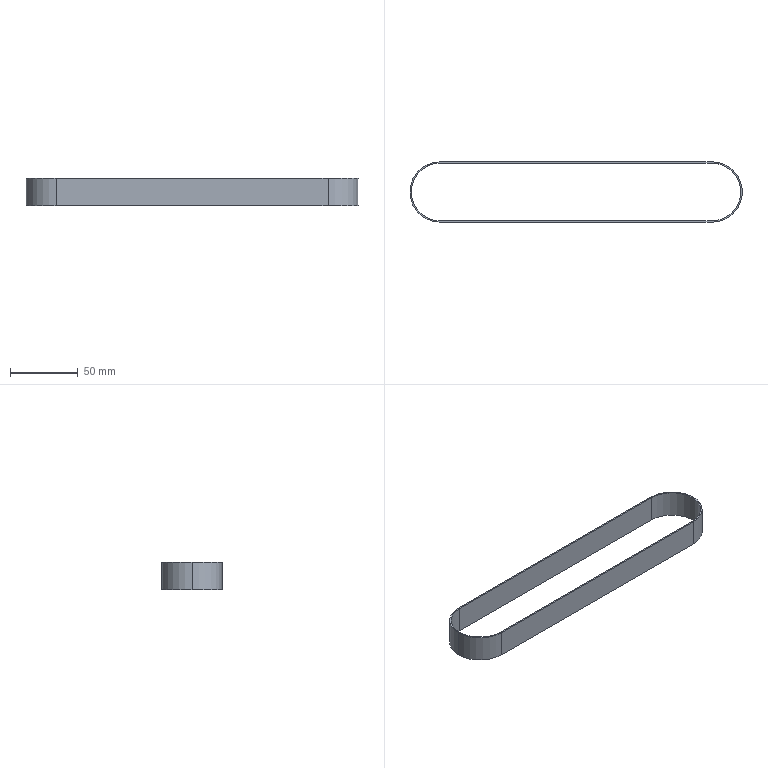Part | STEP file | PN_0049 (timing belt 210L, W20, Z=56) | 1 solid | 12 faces | box 244.45 x 44.45 x 20 mm | volume 10730 mm3 | cylinder 6 | plane 6 | commonest cylinder face diameters 42.45 x3 44.45 x3
STEP:
#1=CARTESIAN_POINT('',(0.,0.,0.));
#2=DIRECTION('',(0.,0.,1.));
#3=DIRECTION('',(1.,0.,0.));
#4=AXIS2_PLACEMENT_3D('',#1,#2,#3);
#5=CARTESIAN_POINT('',(-100.,21.225,10.));
#6=VERTEX_POINT('',#5);
#7=CARTESIAN_POINT('',(-100.,21.225,-10.));
#8=VERTEX_POINT('',#7);
#9=CARTESIAN_POINT('',(-100.,21.225,10.));
#10=DIRECTION('',(0.,0.,-1.));
#11=VECTOR('',#10,1.);
#12=LINE('',#9,#11);
#13=CARTESIAN_POINT('',(-100.,0.,10.));
#14=DIRECTION('',(0.,0.,-1.));
#15=DIRECTION('',(-1.,0.,0.));
#16=AXIS2_PLACEMENT_3D('',#13,#14,#15);
#17=CYLINDRICAL_SURFACE('',#16,21.225);
#18=CARTESIAN_POINT('',(1.571,0.));
#19=DIRECTION('',(0.,1.));
#20=VECTOR('',#19,1.);
#21=LINE('',#18,#20);
#22=(GEOMETRIC_REPRESENTATION_CONTEXT(2)PARAMETRIC_REPRESENTATION_CONTEXT()REPRESENTATION_CONTEXT('',''));
#23=DEFINITIONAL_REPRESENTATION('',(#21),#22);
#24=PCURVE('',#17,#23);
#25=CARTESIAN_POINT('',(-100.,21.225,10.));
#26=DIRECTION('',(0.,-1.,0.));
#27=DIRECTION('',(0.,0.,-1.));
#28=AXIS2_PLACEMENT_3D('',#25,#26,#27);
#29=PLANE('',#28);
#30=CARTESIAN_POINT('',(0.,0.));
#31=DIRECTION('',(1.,0.));
#32=VECTOR('',#31,1.);
#33=LINE('',#30,#32);
#34=(GEOMETRIC_REPRESENTATION_CONTEXT(2)PARAMETRIC_REPRESENTATION_CONTEXT()REPRESENTATION_CONTEXT('',''));
#35=DEFINITIONAL_REPRESENTATION('',(#33),#34);
#36=PCURVE('',#29,#35);
#37=SURFACE_CURVE('',#12,(#24,#36),.PCURVE_S1.);
#38=EDGE_CURVE('',#6,#8,#37,.T.);
#39=ORIENTED_EDGE('',*,*,#38,.T.);
#40=CARTESIAN_POINT('',(-121.225,0.,-10.));
#41=VERTEX_POINT('',#40);
#42=CARTESIAN_POINT('',(-100.,0.,-10.));
#43=DIRECTION('',(0.,0.,1.));
#44=DIRECTION('',(1.,0.,0.));
#45=AXIS2_PLACEMENT_3D('',#42,#43,#44);
#46=CIRCLE('',#45,21.225);
#47=CARTESIAN_POINT('',(3.142,20.));
#48=DIRECTION('',(-1.,0.));
#49=VECTOR('',#48,1.);
#50=LINE('',#47,#49);
#51=(GEOMETRIC_REPRESENTATION_CONTEXT(2)PARAMETRIC_REPRESENTATION_CONTEXT()REPRESENTATION_CONTEXT('',''));
#52=DEFINITIONAL_REPRESENTATION('',(#50),#51);
#53=PCURVE('',#17,#52);
#54=CARTESIAN_POINT('',(-100.,0.,-10.));
#55=DIRECTION('',(0.,0.,1.));
#56=DIRECTION('',(1.,0.,0.));
#57=AXIS2_PLACEMENT_3D('',#54,#55,#56);
#58=PLANE('',#57);
#59=CARTESIAN_POINT('',(0.,0.));
#60=DIRECTION('',(1.,0.));
#61=AXIS2_PLACEMENT_2D('',#59,#60);
#62=CIRCLE('',#61,21.225);
#63=(GEOMETRIC_REPRESENTATION_CONTEXT(2)PARAMETRIC_REPRESENTATION_CONTEXT()REPRESENTATION_CONTEXT('',''));
#64=DEFINITIONAL_REPRESENTATION('',(#62),#63);
#65=PCURVE('',#58,#64);
#66=SURFACE_CURVE('',#46,(#53,#65),.PCURVE_S1.);
#67=EDGE_CURVE('',#8,#41,#66,.T.);
#68=ORIENTED_EDGE('',*,*,#67,.T.);
#69=CARTESIAN_POINT('',(-121.225,0.,10.));
#70=VERTEX_POINT('',#69);
#71=CARTESIAN_POINT('',(-121.225,0.,10.));
#72=DIRECTION('',(0.,0.,-1.));
#73=VECTOR('',#72,1.);
#74=LINE('',#71,#73);
#75=CARTESIAN_POINT('',(0.,0.));
#76=DIRECTION('',(0.,1.));
#77=VECTOR('',#76,1.);
#78=LINE('',#75,#77);
#79=(GEOMETRIC_REPRESENTATION_CONTEXT(2)PARAMETRIC_REPRESENTATION_CONTEXT()REPRESENTATION_CONTEXT('',''));
#80=DEFINITIONAL_REPRESENTATION('',(#78),#79);
#81=PCURVE('',#17,#80);
#82=CARTESIAN_POINT('',(-100.,0.,10.));
#83=DIRECTION('',(0.,0.,-1.));
#84=DIRECTION('',(-1.,0.,0.));
#85=AXIS2_PLACEMENT_3D('',#82,#83,#84);
#86=CYLINDRICAL_SURFACE('',#85,21.225);
#87=CARTESIAN_POINT('',(6.283,0.));
#88=DIRECTION('',(0.,1.));
#89=VECTOR('',#88,1.);
#90=LINE('',#87,#89);
#91=(GEOMETRIC_REPRESENTATION_CONTEXT(2)PARAMETRIC_REPRESENTATION_CONTEXT()REPRESENTATION_CONTEXT('',''));
#92=DEFINITIONAL_REPRESENTATION('',(#90),#91);
#93=PCURVE('',#86,#92);
#94=SURFACE_CURVE('',#74,(#81,#93),.PCURVE_S1.);
#95=EDGE_CURVE('',#70,#41,#94,.T.);
#96=ORIENTED_EDGE('',*,*,#95,.F.);
#97=CARTESIAN_POINT('',(-100.,0.,10.));
#98=DIRECTION('',(0.,0.,1.));
#99=DIRECTION('',(1.,0.,0.));
#100=AXIS2_PLACEMENT_3D('',#97,#98,#99);
#101=CIRCLE('',#100,21.225);
#102=CARTESIAN_POINT('',(3.142,0.));
#103=DIRECTION('',(-1.,0.));
#104=VECTOR('',#103,1.);
#105=LINE('',#102,#104);
#106=(GEOMETRIC_REPRESENTATION_CONTEXT(2)PARAMETRIC_REPRESENTATION_CONTEXT()REPRESENTATION_CONTEXT('',''));
#107=DEFINITIONAL_REPRESENTATION('',(#105),#106);
#108=PCURVE('',#17,#107);
#109=CARTESIAN_POINT('',(-100.,0.,10.));
#110=DIRECTION('',(0.,0.,1.));
#111=DIRECTION('',(1.,0.,0.));
#112=AXIS2_PLACEMENT_3D('',#109,#110,#111);
#113=PLANE('',#112);
#114=CARTESIAN_POINT('',(0.,0.));
#115=DIRECTION('',(1.,0.));
#116=AXIS2_PLACEMENT_2D('',#114,#115);
#117=CIRCLE('',#116,21.225);
#118=(GEOMETRIC_REPRESENTATION_CONTEXT(2)PARAMETRIC_REPRESENTATION_CONTEXT()REPRESENTATION_CONTEXT('',''));
#119=DEFINITIONAL_REPRESENTATION('',(#117),#118);
#120=PCURVE('',#113,#119);
#121=SURFACE_CURVE('',#101,(#108,#120),.PCURVE_S1.);
#122=EDGE_CURVE('',#6,#70,#121,.T.);
#123=ORIENTED_EDGE('',*,*,#122,.F.);
#124=EDGE_LOOP('',(#39,#68,#96,#123));
#125=FACE_BOUND('',#124,.F.);
#126=ADVANCED_FACE('',(#125),#17,.F.);
#127=CARTESIAN_POINT('',(-122.225,0.,10.));
#128=VERTEX_POINT('',#127);
#129=CARTESIAN_POINT('',(-100.,-22.225,10.));
#130=VERTEX_POINT('',#129);
#131=CARTESIAN_POINT('',(-100.,0.,10.));
#132=DIRECTION('',(0.,0.,1.));
#133=DIRECTION('',(1.,0.,0.));
#134=AXIS2_PLACEMENT_3D('',#131,#132,#133);
#135=CIRCLE('',#134,22.225);
#136=CARTESIAN_POINT('',(-100.,0.,10.));
#137=DIRECTION('',(0.,0.,-1.));
#138=DIRECTION('',(-1.,0.,0.));
#139=AXIS2_PLACEMENT_3D('',#136,#137,#138);
#140=CYLINDRICAL_SURFACE('',#139,22.225);
#141=CARTESIAN_POINT('',(9.425,0.));
#142=DIRECTION('',(-1.,0.));
#143=VECTOR('',#142,1.);
#144=LINE('',#141,#143);
#145=(GEOMETRIC_REPRESENTATION_CONTEXT(2)PARAMETRIC_REPRESENTATION_CONTEXT()REPRESENTATION_CONTEXT('',''));
#146=DEFINITIONAL_REPRESENTATION('',(#144),#145);
#147=PCURVE('',#140,#146);
#148=CARTESIAN_POINT('',(0.,0.));
#149=DIRECTION('',(1.,0.));
#150=AXIS2_PLACEMENT_2D('',#148,#149);
#151=CIRCLE('',#150,22.225);
#152=(GEOMETRIC_REPRESENTATION_CONTEXT(2)PARAMETRIC_REPRESENTATION_CONTEXT()REPRESENTATION_CONTEXT('',''));
#153=DEFINITIONAL_REPRESENTATION('',(#151),#152);
#154=PCURVE('',#113,#153);
#155=SURFACE_CURVE('',#135,(#147,#154),.PCURVE_S1.);
#156=EDGE_CURVE('',#128,#130,#155,.T.);
#157=ORIENTED_EDGE('',*,*,#156,.F.);
#158=CARTESIAN_POINT('',(-122.225,0.,-10.));
#159=VERTEX_POINT('',#158);
#160=CARTESIAN_POINT('',(-122.225,0.,10.));
#161=DIRECTION('',(0.,0.,-1.));
#162=VECTOR('',#161,1.);
#163=LINE('',#160,#162);
#164=CARTESIAN_POINT('',(6.283,0.));
#165=DIRECTION('',(0.,1.));
#166=VECTOR('',#165,1.);
#167=LINE('',#164,#166);
#168=(GEOMETRIC_REPRESENTATION_CONTEXT(2)PARAMETRIC_REPRESENTATION_CONTEXT()REPRESENTATION_CONTEXT('',''));
#169=DEFINITIONAL_REPRESENTATION('',(#167),#168);
#170=PCURVE('',#140,#169);
#171=CARTESIAN_POINT('',(-100.,0.,10.));
#172=DIRECTION('',(0.,0.,-1.));
#173=DIRECTION('',(-1.,0.,0.));
#174=AXIS2_PLACEMENT_3D('',#171,#172,#173);
#175=CYLINDRICAL_SURFACE('',#174,22.225);
#176=CARTESIAN_POINT('',(0.,0.));
#177=DIRECTION('',(0.,1.));
#178=VECTOR('',#177,1.);
#179=LINE('',#176,#178);
#180=(GEOMETRIC_REPRESENTATION_CONTEXT(2)PARAMETRIC_REPRESENTATION_CONTEXT()REPRESENTATION_CONTEXT('',''));
#181=DEFINITIONAL_REPRESENTATION('',(#179),#180);
#182=PCURVE('',#175,#181);
#183=SURFACE_CURVE('',#163,(#170,#182),.PCURVE_S1.);
#184=EDGE_CURVE('',#128,#159,#183,.T.);
#185=ORIENTED_EDGE('',*,*,#184,.T.);
#186=CARTESIAN_POINT('',(-100.,-22.225,-10.));
#187=VERTEX_POINT('',#186);
#188=CARTESIAN_POINT('',(-100.,0.,-10.));
#189=DIRECTION('',(0.,0.,1.));
#190=DIRECTION('',(1.,0.,0.));
#191=AXIS2_PLACEMENT_3D('',#188,#189,#190);
#192=CIRCLE('',#191,22.225);
#193=CARTESIAN_POINT('',(9.425,20.));
#194=DIRECTION('',(-1.,0.));
#195=VECTOR('',#194,1.);
#196=LINE('',#193,#195);
#197=(GEOMETRIC_REPRESENTATION_CONTEXT(2)PARAMETRIC_REPRESENTATION_CONTEXT()REPRESENTATION_CONTEXT('',''));
#198=DEFINITIONAL_REPRESENTATION('',(#196),#197);
#199=PCURVE('',#140,#198);
#200=CARTESIAN_POINT('',(0.,0.));
#201=DIRECTION('',(1.,0.));
#202=AXIS2_PLACEMENT_2D('',#200,#201);
#203=CIRCLE('',#202,22.225);
#204=(GEOMETRIC_REPRESENTATION_CONTEXT(2)PARAMETRIC_REPRESENTATION_CONTEXT()REPRESENTATION_CONTEXT('',''));
#205=DEFINITIONAL_REPRESENTATION('',(#203),#204);
#206=PCURVE('',#58,#205);
#207=SURFACE_CURVE('',#192,(#199,#206),.PCURVE_S1.);
#208=EDGE_CURVE('',#159,#187,#207,.T.);
#209=ORIENTED_EDGE('',*,*,#208,.T.);
#210=CARTESIAN_POINT('',(-100.,-22.225,10.));
#211=DIRECTION('',(0.,0.,-1.));
#212=VECTOR('',#211,1.);
#213=LINE('',#210,#212);
#214=CARTESIAN_POINT('',(4.712,0.));
#215=DIRECTION('',(0.,1.));
#216=VECTOR('',#215,1.);
#217=LINE('',#214,#216);
#218=(GEOMETRIC_REPRESENTATION_CONTEXT(2)PARAMETRIC_REPRESENTATION_CONTEXT()REPRESENTATION_CONTEXT('',''));
#219=DEFINITIONAL_REPRESENTATION('',(#217),#218);
#220=PCURVE('',#140,#219);
#221=CARTESIAN_POINT('',(-100.,-22.225,10.));
#222=DIRECTION('',(0.,1.,0.));
#223=DIRECTION('',(0.,0.,1.));
#224=AXIS2_PLACEMENT_3D('',#221,#222,#223);
#225=PLANE('',#224);
#226=CARTESIAN_POINT('',(0.,0.));
#227=DIRECTION('',(-1.,0.));
#228=VECTOR('',#227,1.);
#229=LINE('',#226,#228);
#230=(GEOMETRIC_REPRESENTATION_CONTEXT(2)PARAMETRIC_REPRESENTATION_CONTEXT()REPRESENTATION_CONTEXT('',''));
#231=DEFINITIONAL_REPRESENTATION('',(#229),#230);
#232=PCURVE('',#225,#231);
#233=SURFACE_CURVE('',#213,(#220,#232),.PCURVE_S1.);
#234=EDGE_CURVE('',#130,#187,#233,.T.);
#235=ORIENTED_EDGE('',*,*,#234,.F.);
#236=EDGE_LOOP('',(#157,#185,#209,#235));
#237=FACE_BOUND('',#236,.T.);
#238=ADVANCED_FACE('',(#237),#140,.T.);
#239=CARTESIAN_POINT('',(-100.,22.225,10.));
#240=VERTEX_POINT('',#239);
#241=CARTESIAN_POINT('',(-100.,0.,10.));
#242=DIRECTION('',(0.,0.,1.));
#243=DIRECTION('',(1.,0.,0.));
#244=AXIS2_PLACEMENT_3D('',#241,#242,#243);
#245=CIRCLE('',#244,22.225);
#246=CARTESIAN_POINT('',(0.,0.));
#247=DIRECTION('',(1.,0.));
#248=AXIS2_PLACEMENT_2D('',#246,#247);
#249=CIRCLE('',#248,22.225);
#250=(GEOMETRIC_REPRESENTATION_CONTEXT(2)PARAMETRIC_REPRESENTATION_CONTEXT()REPRESENTATION_CONTEXT('',''));
#251=DEFINITIONAL_REPRESENTATION('',(#249),#250);
#252=PCURVE('',#113,#251);
#253=CARTESIAN_POINT('',(3.142,0.));
#254=DIRECTION('',(-1.,0.));
#255=VECTOR('',#254,1.);
#256=LINE('',#253,#255);
#257=(GEOMETRIC_REPRESENTATION_CONTEXT(2)PARAMETRIC_REPRESENTATION_CONTEXT()REPRESENTATION_CONTEXT('',''));
#258=DEFINITIONAL_REPRESENTATION('',(#256),#257);
#259=PCURVE('',#175,#258);
#260=SURFACE_CURVE('',#245,(#252,#259),.PCURVE_S1.);
#261=EDGE_CURVE('',#240,#128,#260,.T.);
#262=ORIENTED_EDGE('',*,*,#261,.T.);
#263=ORIENTED_EDGE('',*,*,#156,.T.);
#264=CARTESIAN_POINT('',(100.,-22.225,10.));
#265=VERTEX_POINT('',#264);
#266=CARTESIAN_POINT('',(-100.,-22.225,10.));
#267=DIRECTION('',(1.,0.,0.));
#268=VECTOR('',#267,1.);
#269=LINE('',#266,#268);
#270=CARTESIAN_POINT('',(0.,-22.225));
#271=DIRECTION('',(1.,0.));
#272=VECTOR('',#271,1.);
#273=LINE('',#270,#272);
#274=(GEOMETRIC_REPRESENTATION_CONTEXT(2)PARAMETRIC_REPRESENTATION_CONTEXT()REPRESENTATION_CONTEXT('',''));
#275=DEFINITIONAL_REPRESENTATION('',(#273),#274);
#276=PCURVE('',#113,#275);
#277=CARTESIAN_POINT('',(0.,0.));
#278=DIRECTION('',(0.,1.));
#279=VECTOR('',#278,1.);
#280=LINE('',#277,#279);
#281=(GEOMETRIC_REPRESENTATION_CONTEXT(2)PARAMETRIC_REPRESENTATION_CONTEXT()REPRESENTATION_CONTEXT('',''));
#282=DEFINITIONAL_REPRESENTATION('',(#280),#281);
#283=PCURVE('',#225,#282);
#284=SURFACE_CURVE('',#269,(#276,#283),.PCURVE_S1.);
#285=EDGE_CURVE('',#130,#265,#284,.T.);
#286=ORIENTED_EDGE('',*,*,#285,.T.);
#287=CARTESIAN_POINT('',(100.,22.225,10.));
#288=VERTEX_POINT('',#287);
#289=CARTESIAN_POINT('',(100.,0.,10.));
#290=DIRECTION('',(0.,0.,1.));
#291=DIRECTION('',(1.,0.,0.));
#292=AXIS2_PLACEMENT_3D('',#289,#290,#291);
#293=CIRCLE('',#292,22.225);
#294=CARTESIAN_POINT('',(200.,0.));
#295=DIRECTION('',(1.,0.));
#296=AXIS2_PLACEMENT_2D('',#294,#295);
#297=CIRCLE('',#296,22.225);
#298=(GEOMETRIC_REPRESENTATION_CONTEXT(2)PARAMETRIC_REPRESENTATION_CONTEXT()REPRESENTATION_CONTEXT('',''));
#299=DEFINITIONAL_REPRESENTATION('',(#297),#298);
#300=PCURVE('',#113,#299);
#301=CARTESIAN_POINT('',(100.,0.,10.));
#302=DIRECTION('',(0.,0.,-1.));
#303=DIRECTION('',(-1.,0.,0.));
#304=AXIS2_PLACEMENT_3D('',#301,#302,#303);
#305=CYLINDRICAL_SURFACE('',#304,22.225);
#306=CARTESIAN_POINT('',(9.425,0.));
#307=DIRECTION('',(-1.,0.));
#308=VECTOR('',#307,1.);
#309=LINE('',#306,#308);
#310=(GEOMETRIC_REPRESENTATION_CONTEXT(2)PARAMETRIC_REPRESENTATION_CONTEXT()REPRESENTATION_CONTEXT('',''));
#311=DEFINITIONAL_REPRESENTATION('',(#309),#310);
#312=PCURVE('',#305,#311);
#313=SURFACE_CURVE('',#293,(#300,#312),.PCURVE_S1.);
#314=EDGE_CURVE('',#265,#288,#313,.T.);
#315=ORIENTED_EDGE('',*,*,#314,.T.);
#316=CARTESIAN_POINT('',(-100.,22.225,10.));
#317=DIRECTION('',(-1.,0.,0.));
#318=VECTOR('',#317,1.);
#319=LINE('',#316,#318);
#320=CARTESIAN_POINT('',(0.,22.225));
#321=DIRECTION('',(-1.,0.));
#322=VECTOR('',#321,1.);
#323=LINE('',#320,#322);
#324=(GEOMETRIC_REPRESENTATION_CONTEXT(2)PARAMETRIC_REPRESENTATION_CONTEXT()REPRESENTATION_CONTEXT('',''));
#325=DEFINITIONAL_REPRESENTATION('',(#323),#324);
#326=PCURVE('',#113,#325);
#327=CARTESIAN_POINT('',(-100.,22.225,10.));
#328=DIRECTION('',(0.,-1.,0.));
#329=DIRECTION('',(0.,0.,-1.));
#330=AXIS2_PLACEMENT_3D('',#327,#328,#329);
#331=PLANE('',#330);
#332=CARTESIAN_POINT('',(0.,0.));
#333=DIRECTION('',(0.,-1.));
#334=VECTOR('',#333,1.);
#335=LINE('',#332,#334);
#336=(GEOMETRIC_REPRESENTATION_CONTEXT(2)PARAMETRIC_REPRESENTATION_CONTEXT()REPRESENTATION_CONTEXT('',''));
#337=DEFINITIONAL_REPRESENTATION('',(#335),#336);
#338=PCURVE('',#331,#337);
#339=SURFACE_CURVE('',#319,(#326,#338),.PCURVE_S1.);
#340=EDGE_CURVE('',#288,#240,#339,.T.);
#341=ORIENTED_EDGE('',*,*,#340,.T.);
#342=EDGE_LOOP('',(#262,#263,#286,#315,#341));
#343=FACE_BOUND('',#342,.T.);
#344=CARTESIAN_POINT('',(-100.,-21.225,10.));
#345=VERTEX_POINT('',#344);
#346=CARTESIAN_POINT('',(100.,-21.225,10.));
#347=VERTEX_POINT('',#346);
#348=CARTESIAN_POINT('',(-100.,-21.225,10.));
#349=DIRECTION('',(1.,0.,0.));
#350=VECTOR('',#349,1.);
#351=LINE('',#348,#350);
#352=CARTESIAN_POINT('',(0.,-21.225));
#353=DIRECTION('',(1.,0.));
#354=VECTOR('',#353,1.);
#355=LINE('',#352,#354);
#356=(GEOMETRIC_REPRESENTATION_CONTEXT(2)PARAMETRIC_REPRESENTATION_CONTEXT()REPRESENTATION_CONTEXT('',''));
#357=DEFINITIONAL_REPRESENTATION('',(#355),#356);
#358=PCURVE('',#113,#357);
#359=CARTESIAN_POINT('',(-100.,-21.225,10.));
#360=DIRECTION('',(0.,1.,0.));
#361=DIRECTION('',(0.,0.,1.));
#362=AXIS2_PLACEMENT_3D('',#359,#360,#361);
#363=PLANE('',#362);
#364=CARTESIAN_POINT('',(0.,0.));
#365=DIRECTION('',(0.,1.));
#366=VECTOR('',#365,1.);
#367=LINE('',#364,#366);
#368=(GEOMETRIC_REPRESENTATION_CONTEXT(2)PARAMETRIC_REPRESENTATION_CONTEXT()REPRESENTATION_CONTEXT('',''));
#369=DEFINITIONAL_REPRESENTATION('',(#367),#368);
#370=PCURVE('',#363,#369);
#371=SURFACE_CURVE('',#351,(#358,#370),.PCURVE_S1.);
#372=EDGE_CURVE('',#345,#347,#371,.T.);
#373=ORIENTED_EDGE('',*,*,#372,.F.);
#374=CARTESIAN_POINT('',(-100.,0.,10.));
#375=DIRECTION('',(0.,0.,1.));
#376=DIRECTION('',(1.,0.,0.));
#377=AXIS2_PLACEMENT_3D('',#374,#375,#376);
#378=CIRCLE('',#377,21.225);
#379=CARTESIAN_POINT('',(0.,0.));
#380=DIRECTION('',(1.,0.));
#381=AXIS2_PLACEMENT_2D('',#379,#380);
#382=CIRCLE('',#381,21.225);
#383=(GEOMETRIC_REPRESENTATION_CONTEXT(2)PARAMETRIC_REPRESENTATION_CONTEXT()REPRESENTATION_CONTEXT('',''));
#384=DEFINITIONAL_REPRESENTATION('',(#382),#383);
#385=PCURVE('',#113,#384);
#386=CARTESIAN_POINT('',(9.425,0.));
#387=DIRECTION('',(-1.,0.));
#388=VECTOR('',#387,1.);
#389=LINE('',#386,#388);
#390=(GEOMETRIC_REPRESENTATION_CONTEXT(2)PARAMETRIC_REPRESENTATION_CONTEXT()REPRESENTATION_CONTEXT('',''));
#391=DEFINITIONAL_REPRESENTATION('',(#389),#390);
#392=PCURVE('',#86,#391);
#393=SURFACE_CURVE('',#378,(#385,#392),.PCURVE_S1.);
#394=EDGE_CURVE('',#70,#345,#393,.T.);
#395=ORIENTED_EDGE('',*,*,#394,.F.);
#396=ORIENTED_EDGE('',*,*,#122,.F.);
#397=CARTESIAN_POINT('',(100.,21.225,10.));
#398=VERTEX_POINT('',#397);
#399=CARTESIAN_POINT('',(-100.,21.225,10.));
#400=DIRECTION('',(-1.,0.,0.));
#401=VECTOR('',#400,1.);
#402=LINE('',#399,#401);
#403=CARTESIAN_POINT('',(0.,21.225));
#404=DIRECTION('',(-1.,0.));
#405=VECTOR('',#404,1.);
#406=LINE('',#403,#405);
#407=(GEOMETRIC_REPRESENTATION_CONTEXT(2)PARAMETRIC_REPRESENTATION_CONTEXT()REPRESENTATION_CONTEXT('',''));
#408=DEFINITIONAL_REPRESENTATION('',(#406),#407);
#409=PCURVE('',#113,#408);
#410=CARTESIAN_POINT('',(0.,0.));
#411=DIRECTION('',(0.,-1.));
#412=VECTOR('',#411,1.);
#413=LINE('',#410,#412);
#414=(GEOMETRIC_REPRESENTATION_CONTEXT(2)PARAMETRIC_REPRESENTATION_CONTEXT()REPRESENTATION_CONTEXT('',''));
#415=DEFINITIONAL_REPRESENTATION('',(#413),#414);
#416=PCURVE('',#29,#415);
#417=SURFACE_CURVE('',#402,(#409,#416),.PCURVE_S1.);
#418=EDGE_CURVE('',#398,#6,#417,.T.);
#419=ORIENTED_EDGE('',*,*,#418,.F.);
#420=CARTESIAN_POINT('',(100.,0.,10.));
#421=DIRECTION('',(0.,0.,1.));
#422=DIRECTION('',(1.,0.,0.));
#423=AXIS2_PLACEMENT_3D('',#420,#421,#422);
#424=CIRCLE('',#423,21.225);
#425=CARTESIAN_POINT('',(200.,0.));
#426=DIRECTION('',(1.,0.));
#427=AXIS2_PLACEMENT_2D('',#425,#426);
#428=CIRCLE('',#427,21.225);
#429=(GEOMETRIC_REPRESENTATION_CONTEXT(2)PARAMETRIC_REPRESENTATION_CONTEXT()REPRESENTATION_CONTEXT('',''));
#430=DEFINITIONAL_REPRESENTATION('',(#428),#429);
#431=PCURVE('',#113,#430);
#432=CARTESIAN_POINT('',(100.,0.,10.));
#433=DIRECTION('',(0.,0.,-1.));
#434=DIRECTION('',(-1.,0.,0.));
#435=AXIS2_PLACEMENT_3D('',#432,#433,#434);
#436=CYLINDRICAL_SURFACE('',#435,21.225);
#437=CARTESIAN_POINT('',(9.425,0.));
#438=DIRECTION('',(-1.,0.));
#439=VECTOR('',#438,1.);
#440=LINE('',#437,#439);
#441=(GEOMETRIC_REPRESENTATION_CONTEXT(2)PARAMETRIC_REPRESENTATION_CONTEXT()REPRESENTATION_CONTEXT('',''));
#442=DEFINITIONAL_REPRESENTATION('',(#440),#441);
#443=PCURVE('',#436,#442);
#444=SURFACE_CURVE('',#424,(#431,#443),.PCURVE_S1.);
#445=EDGE_CURVE('',#347,#398,#444,.T.);
#446=ORIENTED_EDGE('',*,*,#445,.F.);
#447=EDGE_LOOP('',(#373,#395,#396,#419,#446));
#448=FACE_BOUND('',#447,.T.);
#449=ADVANCED_FACE('',(#343,#448),#113,.T.);
#450=CARTESIAN_POINT('',(-100.,22.225,-10.));
#451=VERTEX_POINT('',#450);
#452=CARTESIAN_POINT('',(-100.,0.,-10.));
#453=DIRECTION('',(0.,0.,1.));
#454=DIRECTION('',(1.,0.,0.));
#455=AXIS2_PLACEMENT_3D('',#452,#453,#454);
#456=CIRCLE('',#455,22.225);
#457=CARTESIAN_POINT('',(0.,0.));
#458=DIRECTION('',(1.,0.));
#459=AXIS2_PLACEMENT_2D('',#457,#458);
#460=CIRCLE('',#459,22.225);
#461=(GEOMETRIC_REPRESENTATION_CONTEXT(2)PARAMETRIC_REPRESENTATION_CONTEXT()REPRESENTATION_CONTEXT('',''));
#462=DEFINITIONAL_REPRESENTATION('',(#460),#461);
#463=PCURVE('',#58,#462);
#464=CARTESIAN_POINT('',(3.142,20.));
#465=DIRECTION('',(-1.,0.));
#466=VECTOR('',#465,1.);
#467=LINE('',#464,#466);
#468=(GEOMETRIC_REPRESENTATION_CONTEXT(2)PARAMETRIC_REPRESENTATION_CONTEXT()REPRESENTATION_CONTEXT('',''));
#469=DEFINITIONAL_REPRESENTATION('',(#467),#468);
#470=PCURVE('',#175,#469);
#471=SURFACE_CURVE('',#456,(#463,#470),.PCURVE_S1.);
#472=EDGE_CURVE('',#451,#159,#471,.T.);
#473=ORIENTED_EDGE('',*,*,#472,.F.);
#474=CARTESIAN_POINT('',(100.,22.225,-10.));
#475=VERTEX_POINT('',#474);
#476=CARTESIAN_POINT('',(-100.,22.225,-10.));
#477=DIRECTION('',(-1.,0.,0.));
#478=VECTOR('',#477,1.);
#479=LINE('',#476,#478);
#480=CARTESIAN_POINT('',(0.,22.225));
#481=DIRECTION('',(-1.,0.));
#482=VECTOR('',#481,1.);
#483=LINE('',#480,#482);
#484=(GEOMETRIC_REPRESENTATION_CONTEXT(2)PARAMETRIC_REPRESENTATION_CONTEXT()REPRESENTATION_CONTEXT('',''));
#485=DEFINITIONAL_REPRESENTATION('',(#483),#484);
#486=PCURVE('',#58,#485);
#487=CARTESIAN_POINT('',(20.,0.));
#488=DIRECTION('',(0.,-1.));
#489=VECTOR('',#488,1.);
#490=LINE('',#487,#489);
#491=(GEOMETRIC_REPRESENTATION_CONTEXT(2)PARAMETRIC_REPRESENTATION_CONTEXT()REPRESENTATION_CONTEXT('',''));
#492=DEFINITIONAL_REPRESENTATION('',(#490),#491);
#493=PCURVE('',#331,#492);
#494=SURFACE_CURVE('',#479,(#486,#493),.PCURVE_S1.);
#495=EDGE_CURVE('',#475,#451,#494,.T.);
#496=ORIENTED_EDGE('',*,*,#495,.F.);
#497=CARTESIAN_POINT('',(100.,-22.225,-10.));
#498=VERTEX_POINT('',#497);
#499=CARTESIAN_POINT('',(100.,0.,-10.));
#500=DIRECTION('',(0.,0.,1.));
#501=DIRECTION('',(1.,0.,0.));
#502=AXIS2_PLACEMENT_3D('',#499,#500,#501);
#503=CIRCLE('',#502,22.225);
#504=CARTESIAN_POINT('',(200.,0.));
#505=DIRECTION('',(1.,0.));
#506=AXIS2_PLACEMENT_2D('',#504,#505);
#507=CIRCLE('',#506,22.225);
#508=(GEOMETRIC_REPRESENTATION_CONTEXT(2)PARAMETRIC_REPRESENTATION_CONTEXT()REPRESENTATION_CONTEXT('',''));
#509=DEFINITIONAL_REPRESENTATION('',(#507),#508);
#510=PCURVE('',#58,#509);
#511=CARTESIAN_POINT('',(9.425,20.));
#512=DIRECTION('',(-1.,0.));
#513=VECTOR('',#512,1.);
#514=LINE('',#511,#513);
#515=(GEOMETRIC_REPRESENTATION_CONTEXT(2)PARAMETRIC_REPRESENTATION_CONTEXT()REPRESENTATION_CONTEXT('',''));
#516=DEFINITIONAL_REPRESENTATION('',(#514),#515);
#517=PCURVE('',#305,#516);
#518=SURFACE_CURVE('',#503,(#510,#517),.PCURVE_S1.);
#519=EDGE_CURVE('',#498,#475,#518,.T.);
#520=ORIENTED_EDGE('',*,*,#519,.F.);
#521=CARTESIAN_POINT('',(-100.,-22.225,-10.));
#522=DIRECTION('',(1.,0.,0.));
#523=VECTOR('',#522,1.);
#524=LINE('',#521,#523);
#525=CARTESIAN_POINT('',(0.,-22.225));
#526=DIRECTION('',(1.,0.));
#527=VECTOR('',#526,1.);
#528=LINE('',#525,#527);
#529=(GEOMETRIC_REPRESENTATION_CONTEXT(2)PARAMETRIC_REPRESENTATION_CONTEXT()REPRESENTATION_CONTEXT('',''));
#530=DEFINITIONAL_REPRESENTATION('',(#528),#529);
#531=PCURVE('',#58,#530);
#532=CARTESIAN_POINT('',(-20.,0.));
#533=DIRECTION('',(0.,1.));
#534=VECTOR('',#533,1.);
#535=LINE('',#532,#534);
#536=(GEOMETRIC_REPRESENTATION_CONTEXT(2)PARAMETRIC_REPRESENTATION_CONTEXT()REPRESENTATION_CONTEXT('',''));
#537=DEFINITIONAL_REPRESENTATION('',(#535),#536);
#538=PCURVE('',#225,#537);
#539=SURFACE_CURVE('',#524,(#531,#538),.PCURVE_S1.);
#540=EDGE_CURVE('',#187,#498,#539,.T.);
#541=ORIENTED_EDGE('',*,*,#540,.F.);
#542=ORIENTED_EDGE('',*,*,#208,.F.);
#543=EDGE_LOOP('',(#473,#496,#520,#541,#542));
#544=FACE_BOUND('',#543,.T.);
#545=ORIENTED_EDGE('',*,*,#67,.T.);
#546=CARTESIAN_POINT('',(-100.,-21.225,-10.));
#547=VERTEX_POINT('',#546);
#548=CARTESIAN_POINT('',(-100.,0.,-10.));
#549=DIRECTION('',(0.,0.,1.));
#550=DIRECTION('',(1.,0.,0.));
#551=AXIS2_PLACEMENT_3D('',#548,#549,#550);
#552=CIRCLE('',#551,21.225);
#553=CARTESIAN_POINT('',(0.,0.));
#554=DIRECTION('',(1.,0.));
#555=AXIS2_PLACEMENT_2D('',#553,#554);
#556=CIRCLE('',#555,21.225);
#557=(GEOMETRIC_REPRESENTATION_CONTEXT(2)PARAMETRIC_REPRESENTATION_CONTEXT()REPRESENTATION_CONTEXT('',''));
#558=DEFINITIONAL_REPRESENTATION('',(#556),#557);
#559=PCURVE('',#58,#558);
#560=CARTESIAN_POINT('',(9.425,20.));
#561=DIRECTION('',(-1.,0.));
#562=VECTOR('',#561,1.);
#563=LINE('',#560,#562);
#564=(GEOMETRIC_REPRESENTATION_CONTEXT(2)PARAMETRIC_REPRESENTATION_CONTEXT()REPRESENTATION_CONTEXT('',''));
#565=DEFINITIONAL_REPRESENTATION('',(#563),#564);
#566=PCURVE('',#86,#565);
#567=SURFACE_CURVE('',#552,(#559,#566),.PCURVE_S1.);
#568=EDGE_CURVE('',#41,#547,#567,.T.);
#569=ORIENTED_EDGE('',*,*,#568,.T.);
#570=CARTESIAN_POINT('',(100.,-21.225,-10.));
#571=VERTEX_POINT('',#570);
#572=CARTESIAN_POINT('',(-100.,-21.225,-10.));
#573=DIRECTION('',(1.,0.,0.));
#574=VECTOR('',#573,1.);
#575=LINE('',#572,#574);
#576=CARTESIAN_POINT('',(0.,-21.225));
#577=DIRECTION('',(1.,0.));
#578=VECTOR('',#577,1.);
#579=LINE('',#576,#578);
#580=(GEOMETRIC_REPRESENTATION_CONTEXT(2)PARAMETRIC_REPRESENTATION_CONTEXT()REPRESENTATION_CONTEXT('',''));
#581=DEFINITIONAL_REPRESENTATION('',(#579),#580);
#582=PCURVE('',#58,#581);
#583=CARTESIAN_POINT('',(-20.,0.));
#584=DIRECTION('',(0.,1.));
#585=VECTOR('',#584,1.);
#586=LINE('',#583,#585);
#587=(GEOMETRIC_REPRESENTATION_CONTEXT(2)PARAMETRIC_REPRESENTATION_CONTEXT()REPRESENTATION_CONTEXT('',''));
#588=DEFINITIONAL_REPRESENTATION('',(#586),#587);
#589=PCURVE('',#363,#588);
#590=SURFACE_CURVE('',#575,(#582,#589),.PCURVE_S1.);
#591=EDGE_CURVE('',#547,#571,#590,.T.);
#592=ORIENTED_EDGE('',*,*,#591,.T.);
#593=CARTESIAN_POINT('',(100.,21.225,-10.));
#594=VERTEX_POINT('',#593);
#595=CARTESIAN_POINT('',(100.,0.,-10.));
#596=DIRECTION('',(0.,0.,1.));
#597=DIRECTION('',(1.,0.,0.));
#598=AXIS2_PLACEMENT_3D('',#595,#596,#597);
#599=CIRCLE('',#598,21.225);
#600=CARTESIAN_POINT('',(200.,0.));
#601=DIRECTION('',(1.,0.));
#602=AXIS2_PLACEMENT_2D('',#600,#601);
#603=CIRCLE('',#602,21.225);
#604=(GEOMETRIC_REPRESENTATION_CONTEXT(2)PARAMETRIC_REPRESENTATION_CONTEXT()REPRESENTATION_CONTEXT('',''));
#605=DEFINITIONAL_REPRESENTATION('',(#603),#604);
#606=PCURVE('',#58,#605);
#607=CARTESIAN_POINT('',(9.425,20.));
#608=DIRECTION('',(-1.,0.));
#609=VECTOR('',#608,1.);
#610=LINE('',#607,#609);
#611=(GEOMETRIC_REPRESENTATION_CONTEXT(2)PARAMETRIC_REPRESENTATION_CONTEXT()REPRESENTATION_CONTEXT('',''));
#612=DEFINITIONAL_REPRESENTATION('',(#610),#611);
#613=PCURVE('',#436,#612);
#614=SURFACE_CURVE('',#599,(#606,#613),.PCURVE_S1.);
#615=EDGE_CURVE('',#571,#594,#614,.T.);
#616=ORIENTED_EDGE('',*,*,#615,.T.);
#617=CARTESIAN_POINT('',(-100.,21.225,-10.));
#618=DIRECTION('',(-1.,0.,0.));
#619=VECTOR('',#618,1.);
#620=LINE('',#617,#619);
#621=CARTESIAN_POINT('',(0.,21.225));
#622=DIRECTION('',(-1.,0.));
#623=VECTOR('',#622,1.);
#624=LINE('',#621,#623);
#625=(GEOMETRIC_REPRESENTATION_CONTEXT(2)PARAMETRIC_REPRESENTATION_CONTEXT()REPRESENTATION_CONTEXT('',''));
#626=DEFINITIONAL_REPRESENTATION('',(#624),#625);
#627=PCURVE('',#58,#626);
#628=CARTESIAN_POINT('',(20.,0.));
#629=DIRECTION('',(0.,-1.));
#630=VECTOR('',#629,1.);
#631=LINE('',#628,#630);
#632=(GEOMETRIC_REPRESENTATION_CONTEXT(2)PARAMETRIC_REPRESENTATION_CONTEXT()REPRESENTATION_CONTEXT('',''));
#633=DEFINITIONAL_REPRESENTATION('',(#631),#632);
#634=PCURVE('',#29,#633);
#635=SURFACE_CURVE('',#620,(#627,#634),.PCURVE_S1.);
#636=EDGE_CURVE('',#594,#8,#635,.T.);
#637=ORIENTED_EDGE('',*,*,#636,.T.);
#638=EDGE_LOOP('',(#545,#569,#592,#616,#637));
#639=FACE_BOUND('',#638,.T.);
#640=ADVANCED_FACE('',(#544,#639),#58,.F.);
#641=ORIENTED_EDGE('',*,*,#184,.F.);
#642=ORIENTED_EDGE('',*,*,#261,.F.);
#643=CARTESIAN_POINT('',(-100.,22.225,10.));
#644=DIRECTION('',(0.,0.,-1.));
#645=VECTOR('',#644,1.);
#646=LINE('',#643,#645);
#647=CARTESIAN_POINT('',(1.571,0.));
#648=DIRECTION('',(0.,1.));
#649=VECTOR('',#648,1.);
#650=LINE('',#647,#649);
#651=(GEOMETRIC_REPRESENTATION_CONTEXT(2)PARAMETRIC_REPRESENTATION_CONTEXT()REPRESENTATION_CONTEXT('',''));
#652=DEFINITIONAL_REPRESENTATION('',(#650),#651);
#653=PCURVE('',#175,#652);
#654=CARTESIAN_POINT('',(0.,0.));
#655=DIRECTION('',(1.,0.));
#656=VECTOR('',#655,1.);
#657=LINE('',#654,#656);
#658=(GEOMETRIC_REPRESENTATION_CONTEXT(2)PARAMETRIC_REPRESENTATION_CONTEXT()REPRESENTATION_CONTEXT('',''));
#659=DEFINITIONAL_REPRESENTATION('',(#657),#658);
#660=PCURVE('',#331,#659);
#661=SURFACE_CURVE('',#646,(#653,#660),.PCURVE_S1.);
#662=EDGE_CURVE('',#240,#451,#661,.T.);
#663=ORIENTED_EDGE('',*,*,#662,.T.);
#664=ORIENTED_EDGE('',*,*,#472,.T.);
#665=EDGE_LOOP('',(#641,#642,#663,#664));
#666=FACE_BOUND('',#665,.T.);
#667=ADVANCED_FACE('',(#666),#175,.T.);
#668=ORIENTED_EDGE('',*,*,#540,.T.);
#669=CARTESIAN_POINT('',(100.,-22.225,10.));
#670=DIRECTION('',(0.,0.,-1.));
#671=VECTOR('',#670,1.);
#672=LINE('',#669,#671);
#673=CARTESIAN_POINT('',(0.,200.));
#674=DIRECTION('',(-1.,0.));
#675=VECTOR('',#674,1.);
#676=LINE('',#673,#675);
#677=(GEOMETRIC_REPRESENTATION_CONTEXT(2)PARAMETRIC_REPRESENTATION_CONTEXT()REPRESENTATION_CONTEXT('',''));
#678=DEFINITIONAL_REPRESENTATION('',(#676),#677);
#679=PCURVE('',#225,#678);
#680=CARTESIAN_POINT('',(4.712,0.));
#681=DIRECTION('',(0.,1.));
#682=VECTOR('',#681,1.);
#683=LINE('',#680,#682);
#684=(GEOMETRIC_REPRESENTATION_CONTEXT(2)PARAMETRIC_REPRESENTATION_CONTEXT()REPRESENTATION_CONTEXT('',''));
#685=DEFINITIONAL_REPRESENTATION('',(#683),#684);
#686=PCURVE('',#305,#685);
#687=SURFACE_CURVE('',#672,(#679,#686),.PCURVE_S1.);
#688=EDGE_CURVE('',#265,#498,#687,.T.);
#689=ORIENTED_EDGE('',*,*,#688,.F.);
#690=ORIENTED_EDGE('',*,*,#285,.F.);
#691=ORIENTED_EDGE('',*,*,#234,.T.);
#692=EDGE_LOOP('',(#668,#689,#690,#691));
#693=FACE_BOUND('',#692,.T.);
#694=ADVANCED_FACE('',(#693),#225,.F.);
#695=ORIENTED_EDGE('',*,*,#519,.T.);
#696=CARTESIAN_POINT('',(100.,22.225,10.));
#697=DIRECTION('',(0.,0.,-1.));
#698=VECTOR('',#697,1.);
#699=LINE('',#696,#698);
#700=CARTESIAN_POINT('',(1.571,0.));
#701=DIRECTION('',(0.,1.));
#702=VECTOR('',#701,1.);
#703=LINE('',#700,#702);
#704=(GEOMETRIC_REPRESENTATION_CONTEXT(2)PARAMETRIC_REPRESENTATION_CONTEXT()REPRESENTATION_CONTEXT('',''));
#705=DEFINITIONAL_REPRESENTATION('',(#703),#704);
#706=PCURVE('',#305,#705);
#707=CARTESIAN_POINT('',(0.,200.));
#708=DIRECTION('',(1.,0.));
#709=VECTOR('',#708,1.);
#710=LINE('',#707,#709);
#711=(GEOMETRIC_REPRESENTATION_CONTEXT(2)PARAMETRIC_REPRESENTATION_CONTEXT()REPRESENTATION_CONTEXT('',''));
#712=DEFINITIONAL_REPRESENTATION('',(#710),#711);
#713=PCURVE('',#331,#712);
#714=SURFACE_CURVE('',#699,(#706,#713),.PCURVE_S1.);
#715=EDGE_CURVE('',#288,#475,#714,.T.);
#716=ORIENTED_EDGE('',*,*,#715,.F.);
#717=ORIENTED_EDGE('',*,*,#314,.F.);
#718=ORIENTED_EDGE('',*,*,#688,.T.);
#719=EDGE_LOOP('',(#695,#716,#717,#718));
#720=FACE_BOUND('',#719,.T.);
#721=ADVANCED_FACE('',(#720),#305,.T.);
#722=ORIENTED_EDGE('',*,*,#495,.T.);
#723=ORIENTED_EDGE('',*,*,#662,.F.);
#724=ORIENTED_EDGE('',*,*,#340,.F.);
#725=ORIENTED_EDGE('',*,*,#715,.T.);
#726=EDGE_LOOP('',(#722,#723,#724,#725));
#727=FACE_BOUND('',#726,.T.);
#728=ADVANCED_FACE('',(#727),#331,.F.);
#729=ORIENTED_EDGE('',*,*,#568,.T.);
#730=CARTESIAN_POINT('',(-100.,-21.225,10.));
#731=DIRECTION('',(0.,0.,-1.));
#732=VECTOR('',#731,1.);
#733=LINE('',#730,#732);
#734=CARTESIAN_POINT('',(4.712,0.));
#735=DIRECTION('',(0.,1.));
#736=VECTOR('',#735,1.);
#737=LINE('',#734,#736);
#738=(GEOMETRIC_REPRESENTATION_CONTEXT(2)PARAMETRIC_REPRESENTATION_CONTEXT()REPRESENTATION_CONTEXT('',''));
#739=DEFINITIONAL_REPRESENTATION('',(#737),#738);
#740=PCURVE('',#86,#739);
#741=CARTESIAN_POINT('',(0.,0.));
#742=DIRECTION('',(-1.,0.));
#743=VECTOR('',#742,1.);
#744=LINE('',#741,#743);
#745=(GEOMETRIC_REPRESENTATION_CONTEXT(2)PARAMETRIC_REPRESENTATION_CONTEXT()REPRESENTATION_CONTEXT('',''));
#746=DEFINITIONAL_REPRESENTATION('',(#744),#745);
#747=PCURVE('',#363,#746);
#748=SURFACE_CURVE('',#733,(#740,#747),.PCURVE_S1.);
#749=EDGE_CURVE('',#345,#547,#748,.T.);
#750=ORIENTED_EDGE('',*,*,#749,.F.);
#751=ORIENTED_EDGE('',*,*,#394,.F.);
#752=ORIENTED_EDGE('',*,*,#95,.T.);
#753=EDGE_LOOP('',(#729,#750,#751,#752));
#754=FACE_BOUND('',#753,.F.);
#755=ADVANCED_FACE('',(#754),#86,.F.);
#756=ORIENTED_EDGE('',*,*,#591,.F.);
#757=ORIENTED_EDGE('',*,*,#749,.F.);
#758=ORIENTED_EDGE('',*,*,#372,.T.);
#759=CARTESIAN_POINT('',(100.,-21.225,10.));
#760=DIRECTION('',(0.,0.,-1.));
#761=VECTOR('',#760,1.);
#762=LINE('',#759,#761);
#763=CARTESIAN_POINT('',(0.,200.));
#764=DIRECTION('',(-1.,0.));
#765=VECTOR('',#764,1.);
#766=LINE('',#763,#765);
#767=(GEOMETRIC_REPRESENTATION_CONTEXT(2)PARAMETRIC_REPRESENTATION_CONTEXT()REPRESENTATION_CONTEXT('',''));
#768=DEFINITIONAL_REPRESENTATION('',(#766),#767);
#769=PCURVE('',#363,#768);
#770=CARTESIAN_POINT('',(4.712,0.));
#771=DIRECTION('',(0.,1.));
#772=VECTOR('',#771,1.);
#773=LINE('',#770,#772);
#774=(GEOMETRIC_REPRESENTATION_CONTEXT(2)PARAMETRIC_REPRESENTATION_CONTEXT()REPRESENTATION_CONTEXT('',''));
#775=DEFINITIONAL_REPRESENTATION('',(#773),#774);
#776=PCURVE('',#436,#775);
#777=SURFACE_CURVE('',#762,(#769,#776),.PCURVE_S1.);
#778=EDGE_CURVE('',#347,#571,#777,.T.);
#779=ORIENTED_EDGE('',*,*,#778,.T.);
#780=EDGE_LOOP('',(#756,#757,#758,#779));
#781=FACE_BOUND('',#780,.T.);
#782=ADVANCED_FACE('',(#781),#363,.T.);
#783=CARTESIAN_POINT('',(100.,21.225,10.));
#784=DIRECTION('',(0.,0.,-1.));
#785=VECTOR('',#784,1.);
#786=LINE('',#783,#785);
#787=CARTESIAN_POINT('',(1.571,0.));
#788=DIRECTION('',(0.,1.));
#789=VECTOR('',#788,1.);
#790=LINE('',#787,#789);
#791=(GEOMETRIC_REPRESENTATION_CONTEXT(2)PARAMETRIC_REPRESENTATION_CONTEXT()REPRESENTATION_CONTEXT('',''));
#792=DEFINITIONAL_REPRESENTATION('',(#790),#791);
#793=PCURVE('',#436,#792);
#794=CARTESIAN_POINT('',(0.,200.));
#795=DIRECTION('',(1.,0.));
#796=VECTOR('',#795,1.);
#797=LINE('',#794,#796);
#798=(GEOMETRIC_REPRESENTATION_CONTEXT(2)PARAMETRIC_REPRESENTATION_CONTEXT()REPRESENTATION_CONTEXT('',''));
#799=DEFINITIONAL_REPRESENTATION('',(#797),#798);
#800=PCURVE('',#29,#799);
#801=SURFACE_CURVE('',#786,(#793,#800),.PCURVE_S1.);
#802=EDGE_CURVE('',#398,#594,#801,.T.);
#803=ORIENTED_EDGE('',*,*,#802,.F.);
#804=ORIENTED_EDGE('',*,*,#445,.F.);
#805=ORIENTED_EDGE('',*,*,#778,.T.);
#806=ORIENTED_EDGE('',*,*,#615,.T.);
#807=EDGE_LOOP('',(#803,#804,#805,#806));
#808=FACE_BOUND('',#807,.F.);
#809=ADVANCED_FACE('',(#808),#436,.F.);
#810=ORIENTED_EDGE('',*,*,#636,.F.);
#811=ORIENTED_EDGE('',*,*,#802,.F.);
#812=ORIENTED_EDGE('',*,*,#418,.T.);
#813=ORIENTED_EDGE('',*,*,#38,.T.);
#814=EDGE_LOOP('',(#810,#811,#812,#813));
#815=FACE_BOUND('',#814,.T.);
#816=ADVANCED_FACE('',(#815),#29,.T.);
#817=CLOSED_SHELL('',(#126,#238,#449,#640,#667,#694,#721,#728,#755,#782,#809,#816));
#818=MANIFOLD_SOLID_BREP('',#817);
#819=(LENGTH_UNIT()NAMED_UNIT(*)SI_UNIT(.MILLI.,.METRE.));
#820=UNCERTAINTY_MEASURE_WITH_UNIT(LENGTH_MEASURE(0.0000001),#819,'','');
#821=(NAMED_UNIT(*)PLANE_ANGLE_UNIT()SI_UNIT($,.RADIAN.));
#822=(NAMED_UNIT(*)SI_UNIT($,.STERADIAN.)SOLID_ANGLE_UNIT());
#823=(GEOMETRIC_REPRESENTATION_CONTEXT(3)GLOBAL_UNCERTAINTY_ASSIGNED_CONTEXT((#820))GLOBAL_UNIT_ASSIGNED_CONTEXT((#819,#821,#822))REPRESENTATION_CONTEXT('',''));
#824=ADVANCED_BREP_SHAPE_REPRESENTATION('',(#4,#818),#823);